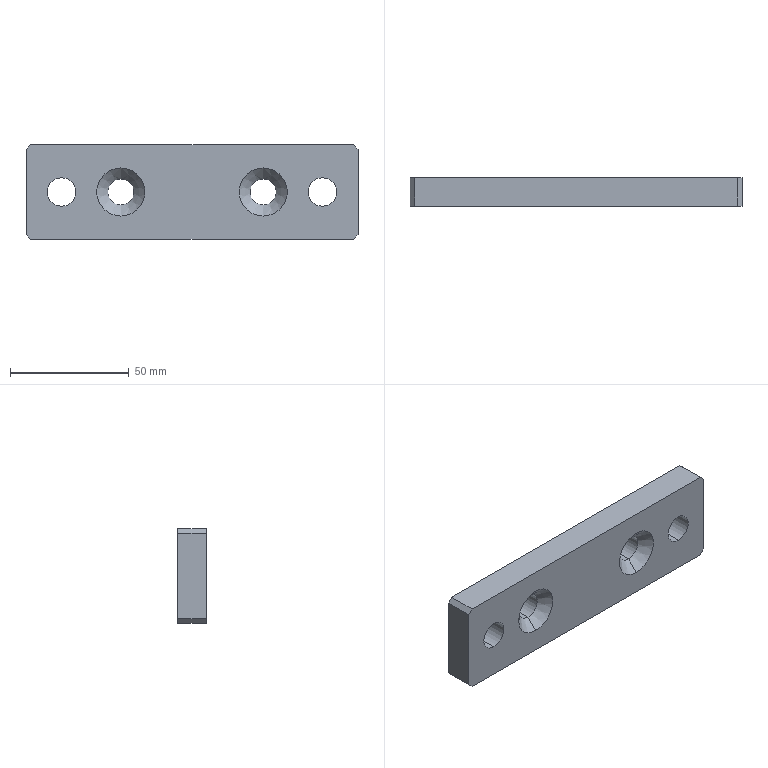Part | SolidWorks | features HoleWzd 2, Chamfer 1, Extrusion 1 | 1 solid | 22 faces | box 140 x 12 x 40 mm | volume 61151 mm3 | plane 10 | cylinder 8 | cone 4 | commonest cylinder face diameters 11 x4 12 x4
STEP:
#1=CARTESIAN_POINT('',(30.,4.65,5.5));
#2=VERTEX_POINT('',#1);
#3=CARTESIAN_POINT('',(30.,4.65,-5.5));
#4=VERTEX_POINT('',#3);
#5=CARTESIAN_POINT('',(30.,4.65,0.));
#6=DIRECTION('',(0.,-1.,0.));
#7=DIRECTION('',(0.,0.,-1.));
#8=AXIS2_PLACEMENT_3D('',#5,#6,#7);
#9=CIRCLE('',#8,5.5);
#10=EDGE_CURVE('',#2,#4,#9,.T.);
#11=ORIENTED_EDGE('',*,*,#10,.F.);
#12=CARTESIAN_POINT('',(30.,0.,10.15));
#13=VERTEX_POINT('',#12);
#14=CARTESIAN_POINT('',(30.,0.,10.15));
#15=DIRECTION('',(0.,-0.7071,0.7071));
#16=VECTOR('',#15,1000.);
#17=LINE('',#14,#16);
#18=EDGE_CURVE('',#2,#13,#17,.T.);
#19=ORIENTED_EDGE('',*,*,#18,.T.);
#20=CARTESIAN_POINT('',(30.,0.,-10.15));
#21=VERTEX_POINT('',#20);
#22=CARTESIAN_POINT('',(30.,0.,0.));
#23=DIRECTION('',(0.,-1.,0.));
#24=DIRECTION('',(0.,0.,-1.));
#25=AXIS2_PLACEMENT_3D('',#22,#23,#24);
#26=CIRCLE('',#25,10.15);
#27=EDGE_CURVE('',#13,#21,#26,.T.);
#28=ORIENTED_EDGE('',*,*,#27,.T.);
#29=CARTESIAN_POINT('',(30.,0.,-10.15));
#30=DIRECTION('',(0.,-0.7071,-0.7071));
#31=VECTOR('',#30,1000.);
#32=LINE('',#29,#31);
#33=EDGE_CURVE('',#4,#21,#32,.T.);
#34=ORIENTED_EDGE('',*,*,#33,.F.);
#35=EDGE_LOOP('',(#11,#19,#28,#34));
#36=FACE_OUTER_BOUND('',#35,.T.);
#37=CARTESIAN_POINT('',(30.,0.,0.));
#38=DIRECTION('',(0.,-1.,0.));
#39=DIRECTION('',(0.,0.,-1.));
#40=AXIS2_PLACEMENT_3D('',#37,#38,#39);
#41=CONICAL_SURFACE('',#40,10.15,0.7854);
#42=ADVANCED_FACE('',(#36),#41,.F.);
#43=CARTESIAN_POINT('',(30.,12.,-5.5));
#44=VERTEX_POINT('',#43);
#45=CARTESIAN_POINT('',(30.,12.,5.5));
#46=VERTEX_POINT('',#45);
#47=CARTESIAN_POINT('',(30.,12.,0.));
#48=DIRECTION('',(0.,1.,0.));
#49=DIRECTION('',(0.,0.,1.));
#50=AXIS2_PLACEMENT_3D('',#47,#48,#49);
#51=CIRCLE('',#50,5.5);
#52=EDGE_CURVE('',#44,#46,#51,.T.);
#53=ORIENTED_EDGE('',*,*,#52,.T.);
#54=CARTESIAN_POINT('',(30.,0.,5.5));
#55=DIRECTION('',(0.,-1.,0.));
#56=VECTOR('',#55,1000.);
#57=LINE('',#54,#56);
#58=EDGE_CURVE('',#46,#2,#57,.T.);
#59=ORIENTED_EDGE('',*,*,#58,.T.);
#60=ORIENTED_EDGE('',*,*,#10,.T.);
#61=CARTESIAN_POINT('',(30.,0.,-5.5));
#62=DIRECTION('',(0.,-1.,0.));
#63=VECTOR('',#62,1000.);
#64=LINE('',#61,#63);
#65=EDGE_CURVE('',#44,#4,#64,.T.);
#66=ORIENTED_EDGE('',*,*,#65,.F.);
#67=EDGE_LOOP('',(#53,#59,#60,#66));
#68=FACE_OUTER_BOUND('',#67,.T.);
#69=CARTESIAN_POINT('',(30.,0.,0.));
#70=DIRECTION('',(0.,-1.,0.));
#71=DIRECTION('',(0.,0.,-1.));
#72=AXIS2_PLACEMENT_3D('',#69,#70,#71);
#73=CYLINDRICAL_SURFACE('',#72,5.5);
#74=ADVANCED_FACE('',(#68),#73,.F.);
#75=CARTESIAN_POINT('',(-30.,4.65,5.5));
#76=VERTEX_POINT('',#75);
#77=CARTESIAN_POINT('',(-30.,4.65,-5.5));
#78=VERTEX_POINT('',#77);
#79=CARTESIAN_POINT('',(-30.,4.65,0.));
#80=DIRECTION('',(0.,-1.,0.));
#81=DIRECTION('',(0.,0.,-1.));
#82=AXIS2_PLACEMENT_3D('',#79,#80,#81);
#83=CIRCLE('',#82,5.5);
#84=EDGE_CURVE('',#76,#78,#83,.T.);
#85=ORIENTED_EDGE('',*,*,#84,.F.);
#86=CARTESIAN_POINT('',(-30.,0.,10.15));
#87=VERTEX_POINT('',#86);
#88=CARTESIAN_POINT('',(-30.,0.,10.15));
#89=DIRECTION('',(0.,-0.7071,0.7071));
#90=VECTOR('',#89,1000.);
#91=LINE('',#88,#90);
#92=EDGE_CURVE('',#76,#87,#91,.T.);
#93=ORIENTED_EDGE('',*,*,#92,.T.);
#94=CARTESIAN_POINT('',(-30.,0.,-10.15));
#95=VERTEX_POINT('',#94);
#96=CARTESIAN_POINT('',(-30.,0.,0.));
#97=DIRECTION('',(0.,-1.,0.));
#98=DIRECTION('',(0.,0.,-1.));
#99=AXIS2_PLACEMENT_3D('',#96,#97,#98);
#100=CIRCLE('',#99,10.15);
#101=EDGE_CURVE('',#87,#95,#100,.T.);
#102=ORIENTED_EDGE('',*,*,#101,.T.);
#103=CARTESIAN_POINT('',(-30.,0.,-10.15));
#104=DIRECTION('',(0.,-0.7071,-0.7071));
#105=VECTOR('',#104,1000.);
#106=LINE('',#103,#105);
#107=EDGE_CURVE('',#78,#95,#106,.T.);
#108=ORIENTED_EDGE('',*,*,#107,.F.);
#109=EDGE_LOOP('',(#85,#93,#102,#108));
#110=FACE_OUTER_BOUND('',#109,.T.);
#111=CARTESIAN_POINT('',(-30.,0.,0.));
#112=DIRECTION('',(0.,-1.,0.));
#113=DIRECTION('',(0.,0.,-1.));
#114=AXIS2_PLACEMENT_3D('',#111,#112,#113);
#115=CONICAL_SURFACE('',#114,10.15,0.7854);
#116=ADVANCED_FACE('',(#110),#115,.F.);
#117=CARTESIAN_POINT('',(-30.,12.,-5.5));
#118=VERTEX_POINT('',#117);
#119=CARTESIAN_POINT('',(-30.,12.,5.5));
#120=VERTEX_POINT('',#119);
#121=CARTESIAN_POINT('',(-30.,12.,0.));
#122=DIRECTION('',(0.,1.,0.));
#123=DIRECTION('',(0.,0.,1.));
#124=AXIS2_PLACEMENT_3D('',#121,#122,#123);
#125=CIRCLE('',#124,5.5);
#126=EDGE_CURVE('',#118,#120,#125,.T.);
#127=ORIENTED_EDGE('',*,*,#126,.T.);
#128=CARTESIAN_POINT('',(-30.,0.,5.5));
#129=DIRECTION('',(0.,-1.,0.));
#130=VECTOR('',#129,1000.);
#131=LINE('',#128,#130);
#132=EDGE_CURVE('',#120,#76,#131,.T.);
#133=ORIENTED_EDGE('',*,*,#132,.T.);
#134=ORIENTED_EDGE('',*,*,#84,.T.);
#135=CARTESIAN_POINT('',(-30.,0.,-5.5));
#136=DIRECTION('',(0.,-1.,0.));
#137=VECTOR('',#136,1000.);
#138=LINE('',#135,#137);
#139=EDGE_CURVE('',#118,#78,#138,.T.);
#140=ORIENTED_EDGE('',*,*,#139,.F.);
#141=EDGE_LOOP('',(#127,#133,#134,#140));
#142=FACE_OUTER_BOUND('',#141,.T.);
#143=CARTESIAN_POINT('',(-30.,0.,0.));
#144=DIRECTION('',(0.,-1.,0.));
#145=DIRECTION('',(0.,0.,-1.));
#146=AXIS2_PLACEMENT_3D('',#143,#144,#145);
#147=CYLINDRICAL_SURFACE('',#146,5.5);
#148=ADVANCED_FACE('',(#142),#147,.F.);
#149=CARTESIAN_POINT('',(-55.,0.,-6.));
#150=VERTEX_POINT('',#149);
#151=CARTESIAN_POINT('',(-55.,0.,6.));
#152=VERTEX_POINT('',#151);
#153=CARTESIAN_POINT('',(-55.,0.,0.));
#154=DIRECTION('',(0.,1.,0.));
#155=DIRECTION('',(0.,0.,1.));
#156=AXIS2_PLACEMENT_3D('',#153,#154,#155);
#157=CIRCLE('',#156,6.);
#158=EDGE_CURVE('',#150,#152,#157,.T.);
#159=ORIENTED_EDGE('',*,*,#158,.F.);
#160=CARTESIAN_POINT('',(-55.,12.,-6.));
#161=VERTEX_POINT('',#160);
#162=CARTESIAN_POINT('',(-55.,12.,-6.));
#163=DIRECTION('',(0.,1.,0.));
#164=VECTOR('',#163,1000.);
#165=LINE('',#162,#164);
#166=EDGE_CURVE('',#150,#161,#165,.T.);
#167=ORIENTED_EDGE('',*,*,#166,.T.);
#168=CARTESIAN_POINT('',(-55.,12.,6.));
#169=VERTEX_POINT('',#168);
#170=CARTESIAN_POINT('',(-55.,12.,0.));
#171=DIRECTION('',(0.,1.,0.));
#172=DIRECTION('',(0.,0.,1.));
#173=AXIS2_PLACEMENT_3D('',#170,#171,#172);
#174=CIRCLE('',#173,6.);
#175=EDGE_CURVE('',#161,#169,#174,.T.);
#176=ORIENTED_EDGE('',*,*,#175,.T.);
#177=CARTESIAN_POINT('',(-55.,12.,6.));
#178=DIRECTION('',(0.,1.,0.));
#179=VECTOR('',#178,1000.);
#180=LINE('',#177,#179);
#181=EDGE_CURVE('',#152,#169,#180,.T.);
#182=ORIENTED_EDGE('',*,*,#181,.F.);
#183=EDGE_LOOP('',(#159,#167,#176,#182));
#184=FACE_OUTER_BOUND('',#183,.T.);
#185=CARTESIAN_POINT('',(-55.,12.,0.));
#186=DIRECTION('',(0.,1.,0.));
#187=DIRECTION('',(0.,0.,1.));
#188=AXIS2_PLACEMENT_3D('',#185,#186,#187);
#189=CYLINDRICAL_SURFACE('',#188,6.);
#190=ADVANCED_FACE('',(#184),#189,.F.);
#191=CARTESIAN_POINT('',(55.,0.,-6.));
#192=VERTEX_POINT('',#191);
#193=CARTESIAN_POINT('',(55.,0.,6.));
#194=VERTEX_POINT('',#193);
#195=CARTESIAN_POINT('',(55.,0.,0.));
#196=DIRECTION('',(0.,1.,0.));
#197=DIRECTION('',(0.,0.,1.));
#198=AXIS2_PLACEMENT_3D('',#195,#196,#197);
#199=CIRCLE('',#198,6.);
#200=EDGE_CURVE('',#192,#194,#199,.T.);
#201=ORIENTED_EDGE('',*,*,#200,.F.);
#202=CARTESIAN_POINT('',(55.,12.,-6.));
#203=VERTEX_POINT('',#202);
#204=CARTESIAN_POINT('',(55.,12.,-6.));
#205=DIRECTION('',(0.,1.,0.));
#206=VECTOR('',#205,1000.);
#207=LINE('',#204,#206);
#208=EDGE_CURVE('',#192,#203,#207,.T.);
#209=ORIENTED_EDGE('',*,*,#208,.T.);
#210=CARTESIAN_POINT('',(55.,12.,6.));
#211=VERTEX_POINT('',#210);
#212=CARTESIAN_POINT('',(55.,12.,0.));
#213=DIRECTION('',(0.,1.,0.));
#214=DIRECTION('',(0.,0.,1.));
#215=AXIS2_PLACEMENT_3D('',#212,#213,#214);
#216=CIRCLE('',#215,6.);
#217=EDGE_CURVE('',#203,#211,#216,.T.);
#218=ORIENTED_EDGE('',*,*,#217,.T.);
#219=CARTESIAN_POINT('',(55.,12.,6.));
#220=DIRECTION('',(0.,1.,0.));
#221=VECTOR('',#220,1000.);
#222=LINE('',#219,#221);
#223=EDGE_CURVE('',#194,#211,#222,.T.);
#224=ORIENTED_EDGE('',*,*,#223,.F.);
#225=EDGE_LOOP('',(#201,#209,#218,#224));
#226=FACE_OUTER_BOUND('',#225,.T.);
#227=CARTESIAN_POINT('',(55.,12.,0.));
#228=DIRECTION('',(0.,1.,0.));
#229=DIRECTION('',(0.,0.,1.));
#230=AXIS2_PLACEMENT_3D('',#227,#228,#229);
#231=CYLINDRICAL_SURFACE('',#230,6.);
#232=ADVANCED_FACE('',(#226),#231,.F.);
#233=CARTESIAN_POINT('',(70.,0.,18.));
#234=VERTEX_POINT('',#233);
#235=CARTESIAN_POINT('',(70.,0.,-18.));
#236=VERTEX_POINT('',#235);
#237=CARTESIAN_POINT('',(70.,0.,-20.));
#238=DIRECTION('',(0.,0.,-1.));
#239=VECTOR('',#238,1000.);
#240=LINE('',#237,#239);
#241=EDGE_CURVE('',#234,#236,#240,.T.);
#242=ORIENTED_EDGE('',*,*,#241,.T.);
#243=CARTESIAN_POINT('',(70.,12.,-18.));
#244=VERTEX_POINT('',#243);
#245=CARTESIAN_POINT('',(70.,12.,-18.));
#246=DIRECTION('',(0.,1.,0.));
#247=VECTOR('',#246,1000.);
#248=LINE('',#245,#247);
#249=EDGE_CURVE('',#236,#244,#248,.T.);
#250=ORIENTED_EDGE('',*,*,#249,.T.);
#251=CARTESIAN_POINT('',(70.,12.,18.));
#252=VERTEX_POINT('',#251);
#253=CARTESIAN_POINT('',(70.,12.,-20.));
#254=DIRECTION('',(0.,0.,-1.));
#255=VECTOR('',#254,1000.);
#256=LINE('',#253,#255);
#257=EDGE_CURVE('',#252,#244,#256,.T.);
#258=ORIENTED_EDGE('',*,*,#257,.F.);
#259=CARTESIAN_POINT('',(70.,12.,18.));
#260=DIRECTION('',(0.,-1.,0.));
#261=VECTOR('',#260,1000.);
#262=LINE('',#259,#261);
#263=EDGE_CURVE('',#252,#234,#262,.T.);
#264=ORIENTED_EDGE('',*,*,#263,.T.);
#265=EDGE_LOOP('',(#242,#250,#258,#264));
#266=FACE_OUTER_BOUND('',#265,.T.);
#267=CARTESIAN_POINT('',(70.,12.,-20.));
#268=DIRECTION('',(-1.,0.,0.));
#269=DIRECTION('',(0.,0.,1.));
#270=AXIS2_PLACEMENT_3D('',#267,#268,#269);
#271=PLANE('',#270);
#272=ADVANCED_FACE('',(#266),#271,.F.);
#273=CARTESIAN_POINT('',(68.,0.,-20.));
#274=VERTEX_POINT('',#273);
#275=CARTESIAN_POINT('',(-68.,0.,-20.));
#276=VERTEX_POINT('',#275);
#277=CARTESIAN_POINT('',(-70.,0.,-20.));
#278=DIRECTION('',(-1.,0.,0.));
#279=VECTOR('',#278,1000.);
#280=LINE('',#277,#279);
#281=EDGE_CURVE('',#274,#276,#280,.T.);
#282=ORIENTED_EDGE('',*,*,#281,.T.);
#283=CARTESIAN_POINT('',(-68.,12.,-20.));
#284=VERTEX_POINT('',#283);
#285=CARTESIAN_POINT('',(-68.,12.,-20.));
#286=DIRECTION('',(0.,1.,0.));
#287=VECTOR('',#286,1000.);
#288=LINE('',#285,#287);
#289=EDGE_CURVE('',#276,#284,#288,.T.);
#290=ORIENTED_EDGE('',*,*,#289,.T.);
#291=CARTESIAN_POINT('',(68.,12.,-20.));
#292=VERTEX_POINT('',#291);
#293=CARTESIAN_POINT('',(-70.,12.,-20.));
#294=DIRECTION('',(-1.,0.,0.));
#295=VECTOR('',#294,1000.);
#296=LINE('',#293,#295);
#297=EDGE_CURVE('',#292,#284,#296,.T.);
#298=ORIENTED_EDGE('',*,*,#297,.F.);
#299=CARTESIAN_POINT('',(68.,12.,-20.));
#300=DIRECTION('',(0.,-1.,0.));
#301=VECTOR('',#300,1000.);
#302=LINE('',#299,#301);
#303=EDGE_CURVE('',#292,#274,#302,.T.);
#304=ORIENTED_EDGE('',*,*,#303,.T.);
#305=EDGE_LOOP('',(#282,#290,#298,#304));
#306=FACE_OUTER_BOUND('',#305,.T.);
#307=CARTESIAN_POINT('',(-70.,12.,-20.));
#308=DIRECTION('',(0.,0.,1.));
#309=DIRECTION('',(1.,0.,0.));
#310=AXIS2_PLACEMENT_3D('',#307,#308,#309);
#311=PLANE('',#310);
#312=ADVANCED_FACE('',(#306),#311,.F.);
#313=CARTESIAN_POINT('',(-70.,0.,-18.));
#314=VERTEX_POINT('',#313);
#315=CARTESIAN_POINT('',(-70.,0.,18.));
#316=VERTEX_POINT('',#315);
#317=CARTESIAN_POINT('',(-70.,0.,-20.));
#318=DIRECTION('',(0.,0.,1.));
#319=VECTOR('',#318,1000.);
#320=LINE('',#317,#319);
#321=EDGE_CURVE('',#314,#316,#320,.T.);
#322=ORIENTED_EDGE('',*,*,#321,.T.);
#323=CARTESIAN_POINT('',(-70.,12.,18.));
#324=VERTEX_POINT('',#323);
#325=CARTESIAN_POINT('',(-70.,12.,18.));
#326=DIRECTION('',(0.,1.,0.));
#327=VECTOR('',#326,1000.);
#328=LINE('',#325,#327);
#329=EDGE_CURVE('',#316,#324,#328,.T.);
#330=ORIENTED_EDGE('',*,*,#329,.T.);
#331=CARTESIAN_POINT('',(-70.,12.,-18.));
#332=VERTEX_POINT('',#331);
#333=CARTESIAN_POINT('',(-70.,12.,-20.));
#334=DIRECTION('',(0.,0.,1.));
#335=VECTOR('',#334,1000.);
#336=LINE('',#333,#335);
#337=EDGE_CURVE('',#332,#324,#336,.T.);
#338=ORIENTED_EDGE('',*,*,#337,.F.);
#339=CARTESIAN_POINT('',(-70.,12.,-18.));
#340=DIRECTION('',(0.,-1.,0.));
#341=VECTOR('',#340,1000.);
#342=LINE('',#339,#341);
#343=EDGE_CURVE('',#332,#314,#342,.T.);
#344=ORIENTED_EDGE('',*,*,#343,.T.);
#345=EDGE_LOOP('',(#322,#330,#338,#344));
#346=FACE_OUTER_BOUND('',#345,.T.);
#347=CARTESIAN_POINT('',(-70.,12.,-20.));
#348=DIRECTION('',(1.,0.,0.));
#349=DIRECTION('',(0.,0.,-1.));
#350=AXIS2_PLACEMENT_3D('',#347,#348,#349);
#351=PLANE('',#350);
#352=ADVANCED_FACE('',(#346),#351,.F.);
#353=CARTESIAN_POINT('',(-68.,12.,20.));
#354=VERTEX_POINT('',#353);
#355=CARTESIAN_POINT('',(68.,12.,20.));
#356=VERTEX_POINT('',#355);
#357=CARTESIAN_POINT('',(-70.,12.,20.));
#358=DIRECTION('',(1.,0.,0.));
#359=VECTOR('',#358,1000.);
#360=LINE('',#357,#359);
#361=EDGE_CURVE('',#354,#356,#360,.T.);
#362=ORIENTED_EDGE('',*,*,#361,.F.);
#363=CARTESIAN_POINT('',(-68.,0.,20.));
#364=VERTEX_POINT('',#363);
#365=CARTESIAN_POINT('',(-68.,12.,20.));
#366=DIRECTION('',(0.,-1.,0.));
#367=VECTOR('',#366,1000.);
#368=LINE('',#365,#367);
#369=EDGE_CURVE('',#354,#364,#368,.T.);
#370=ORIENTED_EDGE('',*,*,#369,.T.);
#371=CARTESIAN_POINT('',(68.,0.,20.));
#372=VERTEX_POINT('',#371);
#373=CARTESIAN_POINT('',(-70.,0.,20.));
#374=DIRECTION('',(1.,0.,0.));
#375=VECTOR('',#374,1000.);
#376=LINE('',#373,#375);
#377=EDGE_CURVE('',#364,#372,#376,.T.);
#378=ORIENTED_EDGE('',*,*,#377,.T.);
#379=CARTESIAN_POINT('',(68.,12.,20.));
#380=DIRECTION('',(0.,1.,0.));
#381=VECTOR('',#380,1000.);
#382=LINE('',#379,#381);
#383=EDGE_CURVE('',#372,#356,#382,.T.);
#384=ORIENTED_EDGE('',*,*,#383,.T.);
#385=EDGE_LOOP('',(#362,#370,#378,#384));
#386=FACE_OUTER_BOUND('',#385,.T.);
#387=CARTESIAN_POINT('',(-70.,12.,20.));
#388=DIRECTION('',(0.,0.,-1.));
#389=DIRECTION('',(-1.,0.,0.));
#390=AXIS2_PLACEMENT_3D('',#387,#388,#389);
#391=PLANE('',#390);
#392=ADVANCED_FACE('',(#386),#391,.F.);
#393=ORIENTED_EDGE('',*,*,#52,.F.);
#394=CARTESIAN_POINT('',(30.,12.,0.));
#395=DIRECTION('',(0.,1.,0.));
#396=DIRECTION('',(0.,0.,1.));
#397=AXIS2_PLACEMENT_3D('',#394,#395,#396);
#398=CIRCLE('',#397,5.5);
#399=EDGE_CURVE('',#46,#44,#398,.T.);
#400=ORIENTED_EDGE('',*,*,#399,.F.);
#401=EDGE_LOOP('',(#393,#400));
#402=FACE_BOUND('',#401,.T.);
#403=ORIENTED_EDGE('',*,*,#126,.F.);
#404=CARTESIAN_POINT('',(-30.,12.,0.));
#405=DIRECTION('',(0.,1.,0.));
#406=DIRECTION('',(0.,0.,1.));
#407=AXIS2_PLACEMENT_3D('',#404,#405,#406);
#408=CIRCLE('',#407,5.5);
#409=EDGE_CURVE('',#120,#118,#408,.T.);
#410=ORIENTED_EDGE('',*,*,#409,.F.);
#411=EDGE_LOOP('',(#403,#410));
#412=FACE_BOUND('',#411,.T.);
#413=CARTESIAN_POINT('',(-55.,12.,0.));
#414=DIRECTION('',(0.,1.,0.));
#415=DIRECTION('',(0.,0.,1.));
#416=AXIS2_PLACEMENT_3D('',#413,#414,#415);
#417=CIRCLE('',#416,6.);
#418=EDGE_CURVE('',#169,#161,#417,.T.);
#419=ORIENTED_EDGE('',*,*,#418,.F.);
#420=ORIENTED_EDGE('',*,*,#175,.F.);
#421=EDGE_LOOP('',(#419,#420));
#422=FACE_BOUND('',#421,.T.);
#423=CARTESIAN_POINT('',(55.,12.,0.));
#424=DIRECTION('',(0.,1.,0.));
#425=DIRECTION('',(0.,0.,1.));
#426=AXIS2_PLACEMENT_3D('',#423,#424,#425);
#427=CIRCLE('',#426,6.);
#428=EDGE_CURVE('',#211,#203,#427,.T.);
#429=ORIENTED_EDGE('',*,*,#428,.F.);
#430=ORIENTED_EDGE('',*,*,#217,.F.);
#431=EDGE_LOOP('',(#429,#430));
#432=FACE_BOUND('',#431,.T.);
#433=ORIENTED_EDGE('',*,*,#337,.T.);
#434=CARTESIAN_POINT('',(-44.,12.,44.));
#435=DIRECTION('',(0.7071,0.,0.7071));
#436=VECTOR('',#435,1000.);
#437=LINE('',#434,#436);
#438=EDGE_CURVE('',#324,#354,#437,.T.);
#439=ORIENTED_EDGE('',*,*,#438,.T.);
#440=ORIENTED_EDGE('',*,*,#361,.T.);
#441=CARTESIAN_POINT('',(44.,12.,44.));
#442=DIRECTION('',(0.7071,0.,-0.7071));
#443=VECTOR('',#442,1000.);
#444=LINE('',#441,#443);
#445=EDGE_CURVE('',#356,#252,#444,.T.);
#446=ORIENTED_EDGE('',*,*,#445,.T.);
#447=ORIENTED_EDGE('',*,*,#257,.T.);
#448=CARTESIAN_POINT('',(44.,12.,-44.));
#449=DIRECTION('',(-0.7071,0.,-0.7071));
#450=VECTOR('',#449,1000.);
#451=LINE('',#448,#450);
#452=EDGE_CURVE('',#244,#292,#451,.T.);
#453=ORIENTED_EDGE('',*,*,#452,.T.);
#454=ORIENTED_EDGE('',*,*,#297,.T.);
#455=CARTESIAN_POINT('',(-44.,12.,-44.));
#456=DIRECTION('',(-0.7071,0.,0.7071));
#457=VECTOR('',#456,1000.);
#458=LINE('',#455,#457);
#459=EDGE_CURVE('',#284,#332,#458,.T.);
#460=ORIENTED_EDGE('',*,*,#459,.T.);
#461=EDGE_LOOP('',(#433,#439,#440,#446,#447,#453,#454,#460));
#462=FACE_OUTER_BOUND('',#461,.T.);
#463=CARTESIAN_POINT('',(0.,12.,0.));
#464=DIRECTION('',(0.,1.,0.));
#465=DIRECTION('',(0.,0.,1.));
#466=AXIS2_PLACEMENT_3D('',#463,#464,#465);
#467=PLANE('',#466);
#468=ADVANCED_FACE('',(#402,#412,#422,#432,#462),#467,.T.);
#469=CARTESIAN_POINT('',(30.,0.,0.));
#470=DIRECTION('',(0.,-1.,0.));
#471=DIRECTION('',(0.,0.,-1.));
#472=AXIS2_PLACEMENT_3D('',#469,#470,#471);
#473=CIRCLE('',#472,10.15);
#474=EDGE_CURVE('',#21,#13,#473,.T.);
#475=ORIENTED_EDGE('',*,*,#474,.F.);
#476=ORIENTED_EDGE('',*,*,#27,.F.);
#477=EDGE_LOOP('',(#475,#476));
#478=FACE_BOUND('',#477,.T.);
#479=CARTESIAN_POINT('',(-30.,0.,0.));
#480=DIRECTION('',(0.,-1.,0.));
#481=DIRECTION('',(0.,0.,-1.));
#482=AXIS2_PLACEMENT_3D('',#479,#480,#481);
#483=CIRCLE('',#482,10.15);
#484=EDGE_CURVE('',#95,#87,#483,.T.);
#485=ORIENTED_EDGE('',*,*,#484,.F.);
#486=ORIENTED_EDGE('',*,*,#101,.F.);
#487=EDGE_LOOP('',(#485,#486));
#488=FACE_BOUND('',#487,.T.);
#489=CARTESIAN_POINT('',(-55.,0.,0.));
#490=DIRECTION('',(0.,1.,0.));
#491=DIRECTION('',(0.,0.,1.));
#492=AXIS2_PLACEMENT_3D('',#489,#490,#491);
#493=CIRCLE('',#492,6.);
#494=EDGE_CURVE('',#152,#150,#493,.T.);
#495=ORIENTED_EDGE('',*,*,#494,.T.);
#496=ORIENTED_EDGE('',*,*,#158,.T.);
#497=EDGE_LOOP('',(#495,#496));
#498=FACE_BOUND('',#497,.T.);
#499=CARTESIAN_POINT('',(55.,0.,0.));
#500=DIRECTION('',(0.,1.,0.));
#501=DIRECTION('',(0.,0.,1.));
#502=AXIS2_PLACEMENT_3D('',#499,#500,#501);
#503=CIRCLE('',#502,6.);
#504=EDGE_CURVE('',#194,#192,#503,.T.);
#505=ORIENTED_EDGE('',*,*,#504,.T.);
#506=ORIENTED_EDGE('',*,*,#200,.T.);
#507=EDGE_LOOP('',(#505,#506));
#508=FACE_BOUND('',#507,.T.);
#509=ORIENTED_EDGE('',*,*,#377,.F.);
#510=CARTESIAN_POINT('',(-68.,0.,20.));
#511=DIRECTION('',(-0.7071,0.,-0.7071));
#512=VECTOR('',#511,1000.);
#513=LINE('',#510,#512);
#514=EDGE_CURVE('',#364,#316,#513,.T.);
#515=ORIENTED_EDGE('',*,*,#514,.T.);
#516=ORIENTED_EDGE('',*,*,#321,.F.);
#517=CARTESIAN_POINT('',(-70.,0.,-18.));
#518=DIRECTION('',(0.7071,0.,-0.7071));
#519=VECTOR('',#518,1000.);
#520=LINE('',#517,#519);
#521=EDGE_CURVE('',#314,#276,#520,.T.);
#522=ORIENTED_EDGE('',*,*,#521,.T.);
#523=ORIENTED_EDGE('',*,*,#281,.F.);
#524=CARTESIAN_POINT('',(68.,0.,-20.));
#525=DIRECTION('',(0.7071,0.,0.7071));
#526=VECTOR('',#525,1000.);
#527=LINE('',#524,#526);
#528=EDGE_CURVE('',#274,#236,#527,.T.);
#529=ORIENTED_EDGE('',*,*,#528,.T.);
#530=ORIENTED_EDGE('',*,*,#241,.F.);
#531=CARTESIAN_POINT('',(70.,0.,18.));
#532=DIRECTION('',(-0.7071,0.,0.7071));
#533=VECTOR('',#532,1000.);
#534=LINE('',#531,#533);
#535=EDGE_CURVE('',#234,#372,#534,.T.);
#536=ORIENTED_EDGE('',*,*,#535,.T.);
#537=EDGE_LOOP('',(#509,#515,#516,#522,#523,#529,#530,#536));
#538=FACE_OUTER_BOUND('',#537,.T.);
#539=CARTESIAN_POINT('',(0.,0.,0.));
#540=DIRECTION('',(0.,1.,0.));
#541=DIRECTION('',(0.,0.,1.));
#542=AXIS2_PLACEMENT_3D('',#539,#540,#541);
#543=PLANE('',#542);
#544=ADVANCED_FACE('',(#478,#488,#498,#508,#538),#543,.F.);
#545=ORIENTED_EDGE('',*,*,#208,.F.);
#546=ORIENTED_EDGE('',*,*,#504,.F.);
#547=ORIENTED_EDGE('',*,*,#223,.T.);
#548=ORIENTED_EDGE('',*,*,#428,.T.);
#549=EDGE_LOOP('',(#545,#546,#547,#548));
#550=FACE_OUTER_BOUND('',#549,.T.);
#551=CARTESIAN_POINT('',(55.,12.,0.));
#552=DIRECTION('',(0.,1.,0.));
#553=DIRECTION('',(0.,0.,1.));
#554=AXIS2_PLACEMENT_3D('',#551,#552,#553);
#555=CYLINDRICAL_SURFACE('',#554,6.);
#556=ADVANCED_FACE('',(#550),#555,.F.);
#557=ORIENTED_EDGE('',*,*,#166,.F.);
#558=ORIENTED_EDGE('',*,*,#494,.F.);
#559=ORIENTED_EDGE('',*,*,#181,.T.);
#560=ORIENTED_EDGE('',*,*,#418,.T.);
#561=EDGE_LOOP('',(#557,#558,#559,#560));
#562=FACE_OUTER_BOUND('',#561,.T.);
#563=CARTESIAN_POINT('',(-55.,12.,0.));
#564=DIRECTION('',(0.,1.,0.));
#565=DIRECTION('',(0.,0.,1.));
#566=AXIS2_PLACEMENT_3D('',#563,#564,#565);
#567=CYLINDRICAL_SURFACE('',#566,6.);
#568=ADVANCED_FACE('',(#562),#567,.F.);
#569=ORIENTED_EDGE('',*,*,#132,.F.);
#570=ORIENTED_EDGE('',*,*,#409,.T.);
#571=ORIENTED_EDGE('',*,*,#139,.T.);
#572=CARTESIAN_POINT('',(-30.,4.65,0.));
#573=DIRECTION('',(0.,-1.,0.));
#574=DIRECTION('',(0.,0.,-1.));
#575=AXIS2_PLACEMENT_3D('',#572,#573,#574);
#576=CIRCLE('',#575,5.5);
#577=EDGE_CURVE('',#78,#76,#576,.T.);
#578=ORIENTED_EDGE('',*,*,#577,.T.);
#579=EDGE_LOOP('',(#569,#570,#571,#578));
#580=FACE_OUTER_BOUND('',#579,.T.);
#581=CARTESIAN_POINT('',(-30.,0.,0.));
#582=DIRECTION('',(0.,-1.,0.));
#583=DIRECTION('',(0.,0.,-1.));
#584=AXIS2_PLACEMENT_3D('',#581,#582,#583);
#585=CYLINDRICAL_SURFACE('',#584,5.5);
#586=ADVANCED_FACE('',(#580),#585,.F.);
#587=ORIENTED_EDGE('',*,*,#92,.F.);
#588=ORIENTED_EDGE('',*,*,#577,.F.);
#589=ORIENTED_EDGE('',*,*,#107,.T.);
#590=ORIENTED_EDGE('',*,*,#484,.T.);
#591=EDGE_LOOP('',(#587,#588,#589,#590));
#592=FACE_OUTER_BOUND('',#591,.T.);
#593=CARTESIAN_POINT('',(-30.,0.,0.));
#594=DIRECTION('',(0.,-1.,0.));
#595=DIRECTION('',(0.,0.,-1.));
#596=AXIS2_PLACEMENT_3D('',#593,#594,#595);
#597=CONICAL_SURFACE('',#596,10.15,0.7854);
#598=ADVANCED_FACE('',(#592),#597,.F.);
#599=ORIENTED_EDGE('',*,*,#58,.F.);
#600=ORIENTED_EDGE('',*,*,#399,.T.);
#601=ORIENTED_EDGE('',*,*,#65,.T.);
#602=CARTESIAN_POINT('',(30.,4.65,0.));
#603=DIRECTION('',(0.,-1.,0.));
#604=DIRECTION('',(0.,0.,-1.));
#605=AXIS2_PLACEMENT_3D('',#602,#603,#604);
#606=CIRCLE('',#605,5.5);
#607=EDGE_CURVE('',#4,#2,#606,.T.);
#608=ORIENTED_EDGE('',*,*,#607,.T.);
#609=EDGE_LOOP('',(#599,#600,#601,#608));
#610=FACE_OUTER_BOUND('',#609,.T.);
#611=CARTESIAN_POINT('',(30.,0.,0.));
#612=DIRECTION('',(0.,-1.,0.));
#613=DIRECTION('',(0.,0.,-1.));
#614=AXIS2_PLACEMENT_3D('',#611,#612,#613);
#615=CYLINDRICAL_SURFACE('',#614,5.5);
#616=ADVANCED_FACE('',(#610),#615,.F.);
#617=ORIENTED_EDGE('',*,*,#18,.F.);
#618=ORIENTED_EDGE('',*,*,#607,.F.);
#619=ORIENTED_EDGE('',*,*,#33,.T.);
#620=ORIENTED_EDGE('',*,*,#474,.T.);
#621=EDGE_LOOP('',(#617,#618,#619,#620));
#622=FACE_OUTER_BOUND('',#621,.T.);
#623=CARTESIAN_POINT('',(30.,0.,0.));
#624=DIRECTION('',(0.,-1.,0.));
#625=DIRECTION('',(0.,0.,-1.));
#626=AXIS2_PLACEMENT_3D('',#623,#624,#625);
#627=CONICAL_SURFACE('',#626,10.15,0.7854);
#628=ADVANCED_FACE('',(#622),#627,.F.);
#629=ORIENTED_EDGE('',*,*,#438,.F.);
#630=ORIENTED_EDGE('',*,*,#329,.F.);
#631=ORIENTED_EDGE('',*,*,#514,.F.);
#632=ORIENTED_EDGE('',*,*,#369,.F.);
#633=EDGE_LOOP('',(#629,#630,#631,#632));
#634=FACE_OUTER_BOUND('',#633,.T.);
#635=CARTESIAN_POINT('',(-68.,12.,20.));
#636=DIRECTION('',(0.7071,0.,-0.7071));
#637=DIRECTION('',(0.,-1.,0.));
#638=AXIS2_PLACEMENT_3D('',#635,#636,#637);
#639=PLANE('',#638);
#640=ADVANCED_FACE('',(#634),#639,.F.);
#641=ORIENTED_EDGE('',*,*,#459,.F.);
#642=ORIENTED_EDGE('',*,*,#289,.F.);
#643=ORIENTED_EDGE('',*,*,#521,.F.);
#644=ORIENTED_EDGE('',*,*,#343,.F.);
#645=EDGE_LOOP('',(#641,#642,#643,#644));
#646=FACE_OUTER_BOUND('',#645,.T.);
#647=CARTESIAN_POINT('',(-70.,12.,-18.));
#648=DIRECTION('',(0.7071,0.,0.7071));
#649=DIRECTION('',(0.,-1.,0.));
#650=AXIS2_PLACEMENT_3D('',#647,#648,#649);
#651=PLANE('',#650);
#652=ADVANCED_FACE('',(#646),#651,.F.);
#653=ORIENTED_EDGE('',*,*,#452,.F.);
#654=ORIENTED_EDGE('',*,*,#249,.F.);
#655=ORIENTED_EDGE('',*,*,#528,.F.);
#656=ORIENTED_EDGE('',*,*,#303,.F.);
#657=EDGE_LOOP('',(#653,#654,#655,#656));
#658=FACE_OUTER_BOUND('',#657,.T.);
#659=CARTESIAN_POINT('',(68.,12.,-20.));
#660=DIRECTION('',(-0.7071,0.,0.7071));
#661=DIRECTION('',(0.,-1.,0.));
#662=AXIS2_PLACEMENT_3D('',#659,#660,#661);
#663=PLANE('',#662);
#664=ADVANCED_FACE('',(#658),#663,.F.);
#665=ORIENTED_EDGE('',*,*,#445,.F.);
#666=ORIENTED_EDGE('',*,*,#383,.F.);
#667=ORIENTED_EDGE('',*,*,#535,.F.);
#668=ORIENTED_EDGE('',*,*,#263,.F.);
#669=EDGE_LOOP('',(#665,#666,#667,#668));
#670=FACE_OUTER_BOUND('',#669,.T.);
#671=CARTESIAN_POINT('',(70.,12.,18.));
#672=DIRECTION('',(-0.7071,0.,-0.7071));
#673=DIRECTION('',(0.,-1.,0.));
#674=AXIS2_PLACEMENT_3D('',#671,#672,#673);
#675=PLANE('',#674);
#676=ADVANCED_FACE('',(#670),#675,.F.);
#677=CLOSED_SHELL('',(#42,#74,#116,#148,#190,#232,#272,#312,#352,#392,#468,#544,#556,#568,#586,#598,#616,#628,#640,#652,#664,#676));
#678=MANIFOLD_SOLID_BREP('',#677);
#679=CARTESIAN_POINT('',(0.,0.,0.));
#680=DIRECTION('',(0.,0.,1.));
#681=DIRECTION('',(1.,0.,0.));
#682=AXIS2_PLACEMENT_3D('',#679,#680,#681);
#683=(LENGTH_UNIT()NAMED_UNIT(*)SI_UNIT(.MILLI.,.METRE.));
#684=UNCERTAINTY_MEASURE_WITH_UNIT(LENGTH_MEASURE(0.00001),#683,'','');
#685=(NAMED_UNIT(*)PLANE_ANGLE_UNIT()SI_UNIT($,.RADIAN.));
#686=(NAMED_UNIT(*)SI_UNIT($,.STERADIAN.)SOLID_ANGLE_UNIT());
#687=(GEOMETRIC_REPRESENTATION_CONTEXT(3)GLOBAL_UNCERTAINTY_ASSIGNED_CONTEXT((#684))GLOBAL_UNIT_ASSIGNED_CONTEXT((#683,#685,#686))REPRESENTATION_CONTEXT('',''));
#688=ADVANCED_BREP_SHAPE_REPRESENTATION('',(#678,#682),#687);